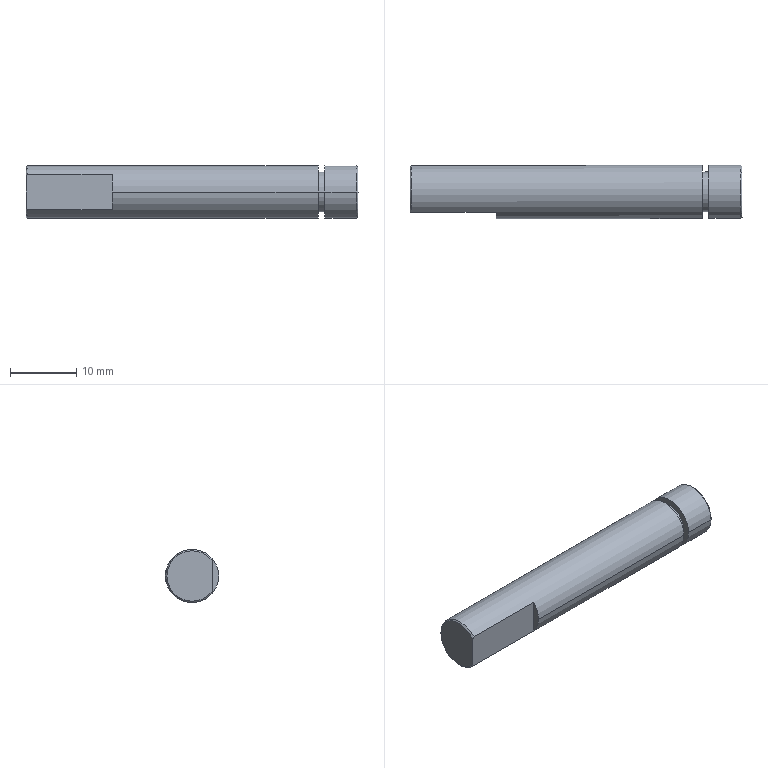Part | SolidWorks | features BaseBody 1 | 1 solid | 15 faces | box 50.007 x 8.035 x 8 mm | volume 2443 mm3 | cylinder 6 | plane 6 | cone 3 | commonest cylinder face diameters 8 x4 6 x2
STEP:
#1=CARTESIAN_POINT('',(349.379,469.971,106.919));
#2=VERTEX_POINT('',#1);
#3=CARTESIAN_POINT('',(349.387,461.971,106.919));
#4=VERTEX_POINT('',#3);
#5=CARTESIAN_POINT('',(349.383,465.971,106.919));
#6=DIRECTION('',(-1.,-0.0009599,0.));
#7=DIRECTION('',(0.0009599,-1.,0.));
#8=AXIS2_PLACEMENT_3D('',#5,#6,#7);
#9=CIRCLE('',#8,4.);
#10=EDGE_CURVE('',#2,#4,#9,.T.);
#11=ORIENTED_EDGE('',*,*,#10,.F.);
#12=CARTESIAN_POINT('',(354.179,469.976,106.919));
#13=VERTEX_POINT('',#12);
#14=CARTESIAN_POINT('',(304.379,469.928,106.919));
#15=DIRECTION('',(1.,0.0009599,0.));
#16=VECTOR('',#15,1000.);
#17=LINE('',#14,#16);
#18=EDGE_CURVE('',#2,#13,#17,.T.);
#19=ORIENTED_EDGE('',*,*,#18,.T.);
#20=CARTESIAN_POINT('',(354.187,461.976,106.919));
#21=VERTEX_POINT('',#20);
#22=CARTESIAN_POINT('',(354.183,465.976,106.919));
#23=DIRECTION('',(1.,0.0009599,0.));
#24=DIRECTION('',(-0.0009599,1.,0.));
#25=AXIS2_PLACEMENT_3D('',#22,#23,#24);
#26=CIRCLE('',#25,4.);
#27=EDGE_CURVE('',#21,#13,#26,.T.);
#28=ORIENTED_EDGE('',*,*,#27,.F.);
#29=CARTESIAN_POINT('',(304.387,461.928,106.919));
#30=DIRECTION('',(1.,0.0009599,0.));
#31=VECTOR('',#30,1000.);
#32=LINE('',#29,#31);
#33=EDGE_CURVE('',#4,#21,#32,.T.);
#34=ORIENTED_EDGE('',*,*,#33,.F.);
#35=EDGE_LOOP('',(#11,#19,#28,#34));
#36=FACE_OUTER_BOUND('',#35,.T.);
#37=CARTESIAN_POINT('',(304.383,465.928,106.919));
#38=DIRECTION('',(1.,0.0009599,0.));
#39=DIRECTION('',(0.0009599,-1.,0.));
#40=AXIS2_PLACEMENT_3D('',#37,#38,#39);
#41=CYLINDRICAL_SURFACE('',#40,4.);
#42=ADVANCED_FACE('',(#36),#41,.T.);
#43=CARTESIAN_POINT('',(348.38,468.97,106.919));
#44=VERTEX_POINT('',#43);
#45=CARTESIAN_POINT('',(348.386,462.97,106.919));
#46=VERTEX_POINT('',#45);
#47=CARTESIAN_POINT('',(348.383,465.97,106.919));
#48=DIRECTION('',(-1.,-0.0009599,0.));
#49=DIRECTION('',(-0.0009599,1.,0.));
#50=AXIS2_PLACEMENT_3D('',#47,#48,#49);
#51=CIRCLE('',#50,3.);
#52=EDGE_CURVE('',#44,#46,#51,.T.);
#53=ORIENTED_EDGE('',*,*,#52,.F.);
#54=CARTESIAN_POINT('',(349.38,468.971,106.919));
#55=VERTEX_POINT('',#54);
#56=CARTESIAN_POINT('',(354.38,468.976,106.919));
#57=DIRECTION('',(1.,0.0009599,0.));
#58=VECTOR('',#57,1000.);
#59=LINE('',#56,#58);
#60=EDGE_CURVE('',#44,#55,#59,.T.);
#61=ORIENTED_EDGE('',*,*,#60,.T.);
#62=CARTESIAN_POINT('',(349.386,462.971,106.919));
#63=VERTEX_POINT('',#62);
#64=CARTESIAN_POINT('',(349.383,465.971,106.919));
#65=DIRECTION('',(1.,0.0009599,0.));
#66=DIRECTION('',(-0.0009599,1.,0.));
#67=AXIS2_PLACEMENT_3D('',#64,#65,#66);
#68=CIRCLE('',#67,3.);
#69=EDGE_CURVE('',#63,#55,#68,.T.);
#70=ORIENTED_EDGE('',*,*,#69,.F.);
#71=CARTESIAN_POINT('',(354.386,462.976,106.919));
#72=DIRECTION('',(1.,0.0009599,0.));
#73=VECTOR('',#72,1000.);
#74=LINE('',#71,#73);
#75=EDGE_CURVE('',#46,#63,#74,.T.);
#76=ORIENTED_EDGE('',*,*,#75,.F.);
#77=EDGE_LOOP('',(#53,#61,#70,#76));
#78=FACE_OUTER_BOUND('',#77,.T.);
#79=CARTESIAN_POINT('',(354.383,465.976,106.919));
#80=DIRECTION('',(1.,0.0009599,0.));
#81=DIRECTION('',(0.0009599,-1.,0.));
#82=AXIS2_PLACEMENT_3D('',#79,#80,#81);
#83=CYLINDRICAL_SURFACE('',#82,3.);
#84=ADVANCED_FACE('',(#78),#83,.T.);
#85=CARTESIAN_POINT('',(304.579,469.928,106.919));
#86=VERTEX_POINT('',#85);
#87=CARTESIAN_POINT('',(304.586,462.928,104.273));
#88=VERTEX_POINT('',#87);
#89=CARTESIAN_POINT('',(304.583,465.928,106.919));
#90=DIRECTION('',(-1.,-0.0009599,0.));
#91=DIRECTION('',(-0.0009599,1.,0.));
#92=AXIS2_PLACEMENT_3D('',#89,#90,#91);
#93=CIRCLE('',#92,4.);
#94=EDGE_CURVE('',#86,#88,#93,.T.);
#95=ORIENTED_EDGE('',*,*,#94,.F.);
#96=CARTESIAN_POINT('',(348.379,469.97,106.919));
#97=VERTEX_POINT('',#96);
#98=CARTESIAN_POINT('',(304.379,469.928,106.919));
#99=DIRECTION('',(1.,0.0009599,0.));
#100=VECTOR('',#99,1000.);
#101=LINE('',#98,#100);
#102=EDGE_CURVE('',#86,#97,#101,.T.);
#103=ORIENTED_EDGE('',*,*,#102,.T.);
#104=CARTESIAN_POINT('',(348.387,461.97,106.919));
#105=VERTEX_POINT('',#104);
#106=CARTESIAN_POINT('',(348.383,465.97,106.919));
#107=DIRECTION('',(1.,0.0009599,0.));
#108=DIRECTION('',(-0.0009599,1.,0.));
#109=AXIS2_PLACEMENT_3D('',#106,#107,#108);
#110=CIRCLE('',#109,4.);
#111=EDGE_CURVE('',#105,#97,#110,.T.);
#112=ORIENTED_EDGE('',*,*,#111,.F.);
#113=CARTESIAN_POINT('',(317.387,461.941,106.919));
#114=VERTEX_POINT('',#113);
#115=CARTESIAN_POINT('',(304.387,461.928,106.919));
#116=DIRECTION('',(1.,0.0009599,0.));
#117=VECTOR('',#116,1000.);
#118=LINE('',#115,#117);
#119=EDGE_CURVE('',#114,#105,#118,.T.);
#120=ORIENTED_EDGE('',*,*,#119,.F.);
#121=CARTESIAN_POINT('',(317.386,462.941,104.273));
#122=VERTEX_POINT('',#121);
#123=CARTESIAN_POINT('',(317.383,465.941,106.919));
#124=DIRECTION('',(-1.,-0.0009599,0.));
#125=DIRECTION('',(0.0007199,-0.75,-0.6614));
#126=AXIS2_PLACEMENT_3D('',#123,#124,#125);
#127=CIRCLE('',#126,4.);
#128=EDGE_CURVE('',#122,#114,#127,.T.);
#129=ORIENTED_EDGE('',*,*,#128,.F.);
#130=CARTESIAN_POINT('',(317.386,462.941,104.273));
#131=DIRECTION('',(-1.,-0.0009599,0.));
#132=VECTOR('',#131,1000.);
#133=LINE('',#130,#132);
#134=EDGE_CURVE('',#122,#88,#133,.T.);
#135=ORIENTED_EDGE('',*,*,#134,.T.);
#136=EDGE_LOOP('',(#95,#103,#112,#120,#129,#135));
#137=FACE_OUTER_BOUND('',#136,.T.);
#138=CARTESIAN_POINT('',(304.383,465.928,106.919));
#139=DIRECTION('',(1.,0.0009599,0.));
#140=DIRECTION('',(0.0009599,-1.,0.));
#141=AXIS2_PLACEMENT_3D('',#138,#139,#140);
#142=CYLINDRICAL_SURFACE('',#141,4.);
#143=ADVANCED_FACE('',(#137),#142,.T.);
#144=CARTESIAN_POINT('',(354.386,462.176,106.919));
#145=VERTEX_POINT('',#144);
#146=CARTESIAN_POINT('',(354.379,469.776,106.919));
#147=VERTEX_POINT('',#146);
#148=CARTESIAN_POINT('',(354.383,465.976,106.919));
#149=DIRECTION('',(1.,0.0009599,0.));
#150=DIRECTION('',(0.0009599,-1.,0.));
#151=AXIS2_PLACEMENT_3D('',#148,#149,#150);
#152=CIRCLE('',#151,3.8);
#153=EDGE_CURVE('',#145,#147,#152,.T.);
#154=ORIENTED_EDGE('',*,*,#153,.F.);
#155=CARTESIAN_POINT('',(354.286,462.076,106.919));
#156=DIRECTION('',(-0.7064,-0.7078,0.));
#157=VECTOR('',#156,1000.);
#158=LINE('',#155,#157);
#159=EDGE_CURVE('',#145,#21,#158,.T.);
#160=ORIENTED_EDGE('',*,*,#159,.T.);
#161=ORIENTED_EDGE('',*,*,#27,.T.);
#162=CARTESIAN_POINT('',(354.279,469.876,106.919));
#163=DIRECTION('',(-0.7078,0.7064,0.));
#164=VECTOR('',#163,1000.);
#165=LINE('',#162,#164);
#166=EDGE_CURVE('',#147,#13,#165,.T.);
#167=ORIENTED_EDGE('',*,*,#166,.F.);
#168=EDGE_LOOP('',(#154,#160,#161,#167));
#169=FACE_OUTER_BOUND('',#168,.T.);
#170=CARTESIAN_POINT('',(354.283,465.976,106.919));
#171=DIRECTION('',(-1.,-0.0009599,0.));
#172=DIRECTION('',(-0.0009599,1.,0.));
#173=AXIS2_PLACEMENT_3D('',#170,#171,#172);
#174=CONICAL_SURFACE('',#173,3.9,0.7854);
#175=ADVANCED_FACE('',(#169),#174,.T.);
#176=CARTESIAN_POINT('',(354.383,465.976,106.919));
#177=DIRECTION('',(1.,0.0009599,0.));
#178=DIRECTION('',(0.0009599,-1.,0.));
#179=AXIS2_PLACEMENT_3D('',#176,#177,#178);
#180=CIRCLE('',#179,3.8);
#181=EDGE_CURVE('',#147,#145,#180,.T.);
#182=ORIENTED_EDGE('',*,*,#181,.T.);
#183=ORIENTED_EDGE('',*,*,#153,.T.);
#184=EDGE_LOOP('',(#182,#183));
#185=FACE_OUTER_BOUND('',#184,.T.);
#186=CARTESIAN_POINT('',(354.383,465.976,106.919));
#187=DIRECTION('',(-1.,-0.0009599,0.));
#188=DIRECTION('',(-0.0009599,1.,0.));
#189=AXIS2_PLACEMENT_3D('',#186,#187,#188);
#190=PLANE('',#189);
#191=ADVANCED_FACE('',(#185),#190,.F.);
#192=ORIENTED_EDGE('',*,*,#159,.F.);
#193=ORIENTED_EDGE('',*,*,#181,.F.);
#194=ORIENTED_EDGE('',*,*,#166,.T.);
#195=CARTESIAN_POINT('',(354.183,465.976,106.919));
#196=DIRECTION('',(1.,0.0009599,0.));
#197=DIRECTION('',(-0.0009599,1.,0.));
#198=AXIS2_PLACEMENT_3D('',#195,#196,#197);
#199=CIRCLE('',#198,4.);
#200=EDGE_CURVE('',#13,#21,#199,.T.);
#201=ORIENTED_EDGE('',*,*,#200,.T.);
#202=EDGE_LOOP('',(#192,#193,#194,#201));
#203=FACE_OUTER_BOUND('',#202,.T.);
#204=CARTESIAN_POINT('',(354.283,465.976,106.919));
#205=DIRECTION('',(-1.,-0.0009599,0.));
#206=DIRECTION('',(-0.0009599,1.,0.));
#207=AXIS2_PLACEMENT_3D('',#204,#205,#206);
#208=CONICAL_SURFACE('',#207,3.9,0.7854);
#209=ADVANCED_FACE('',(#203),#208,.T.);
#210=ORIENTED_EDGE('',*,*,#128,.T.);
#211=CARTESIAN_POINT('',(317.386,462.941,109.565));
#212=VERTEX_POINT('',#211);
#213=CARTESIAN_POINT('',(317.383,465.941,106.919));
#214=DIRECTION('',(-1.,-0.0009599,0.));
#215=DIRECTION('',(0.0007199,-0.75,-0.6614));
#216=AXIS2_PLACEMENT_3D('',#213,#214,#215);
#217=CIRCLE('',#216,4.);
#218=EDGE_CURVE('',#114,#212,#217,.T.);
#219=ORIENTED_EDGE('',*,*,#218,.T.);
#220=CARTESIAN_POINT('',(317.386,462.941,104.273));
#221=DIRECTION('',(0.,0.,1.));
#222=VECTOR('',#221,1000.);
#223=LINE('',#220,#222);
#224=EDGE_CURVE('',#122,#212,#223,.T.);
#225=ORIENTED_EDGE('',*,*,#224,.F.);
#226=EDGE_LOOP('',(#210,#219,#225));
#227=FACE_OUTER_BOUND('',#226,.T.);
#228=CARTESIAN_POINT('',(317.383,465.941,106.919));
#229=DIRECTION('',(-1.,-0.0009599,0.));
#230=DIRECTION('',(-0.0009599,1.,0.));
#231=AXIS2_PLACEMENT_3D('',#228,#229,#230);
#232=PLANE('',#231);
#233=ADVANCED_FACE('',(#227),#232,.T.);
#234=CARTESIAN_POINT('',(304.386,462.928,109.252));
#235=VERTEX_POINT('',#234);
#236=CARTESIAN_POINT('',(304.386,462.928,104.587));
#237=VERTEX_POINT('',#236);
#238=CARTESIAN_POINT('',(304.383,465.928,106.919));
#239=DIRECTION('',(-1.,-0.0009599,0.));
#240=DIRECTION('',(0.0007578,-0.7895,0.6138));
#241=AXIS2_PLACEMENT_3D('',#238,#239,#240);
#242=CIRCLE('',#241,3.8);
#243=EDGE_CURVE('',#235,#237,#242,.T.);
#244=ORIENTED_EDGE('',*,*,#243,.T.);
#245=CARTESIAN_POINT('',(304.386,462.928,104.587));
#246=DIRECTION('',(0.,0.,1.));
#247=VECTOR('',#246,1000.);
#248=LINE('',#245,#247);
#249=EDGE_CURVE('',#237,#235,#248,.T.);
#250=ORIENTED_EDGE('',*,*,#249,.T.);
#251=EDGE_LOOP('',(#244,#250));
#252=FACE_OUTER_BOUND('',#251,.T.);
#253=CARTESIAN_POINT('',(304.383,465.928,106.919));
#254=DIRECTION('',(-1.,-0.0009599,0.));
#255=DIRECTION('',(-0.0009599,1.,0.));
#256=AXIS2_PLACEMENT_3D('',#253,#254,#255);
#257=PLANE('',#256);
#258=ADVANCED_FACE('',(#252),#257,.T.);
#259=CARTESIAN_POINT('',(304.586,462.928,104.273));
#260=CARTESIAN_POINT('',(304.562,462.928,104.308));
#261=CARTESIAN_POINT('',(304.517,462.928,104.378));
#262=CARTESIAN_POINT('',(304.45,462.928,104.483));
#263=CARTESIAN_POINT('',(304.407,462.928,104.552));
#264=CARTESIAN_POINT('',(304.386,462.928,104.587));
#265=B_SPLINE_CURVE_WITH_KNOTS('',3,(#259,#260,#261,#262,#263,#264),.UNSPECIFIED.,.F.,.F.,(4,1,1,4),(0.,0.3333,0.6667,1.),.UNSPECIFIED.);
#266=EDGE_CURVE('',#88,#237,#265,.T.);
#267=ORIENTED_EDGE('',*,*,#266,.F.);
#268=ORIENTED_EDGE('',*,*,#134,.F.);
#269=ORIENTED_EDGE('',*,*,#224,.T.);
#270=CARTESIAN_POINT('',(304.586,462.928,109.565));
#271=VERTEX_POINT('',#270);
#272=CARTESIAN_POINT('',(304.586,462.928,109.565));
#273=DIRECTION('',(1.,0.0009599,0.));
#274=VECTOR('',#273,1000.);
#275=LINE('',#272,#274);
#276=EDGE_CURVE('',#271,#212,#275,.T.);
#277=ORIENTED_EDGE('',*,*,#276,.F.);
#278=CARTESIAN_POINT('',(304.386,462.928,109.252));
#279=CARTESIAN_POINT('',(304.407,462.928,109.286));
#280=CARTESIAN_POINT('',(304.45,462.928,109.356));
#281=CARTESIAN_POINT('',(304.517,462.928,109.46));
#282=CARTESIAN_POINT('',(304.562,462.928,109.53));
#283=CARTESIAN_POINT('',(304.586,462.928,109.565));
#284=B_SPLINE_CURVE_WITH_KNOTS('',3,(#278,#279,#280,#281,#282,#283),.UNSPECIFIED.,.F.,.F.,(4,1,1,4),(0.,0.3333,0.6667,1.),.UNSPECIFIED.);
#285=EDGE_CURVE('',#235,#271,#284,.T.);
#286=ORIENTED_EDGE('',*,*,#285,.F.);
#287=ORIENTED_EDGE('',*,*,#249,.F.);
#288=EDGE_LOOP('',(#267,#268,#269,#277,#286,#287));
#289=FACE_OUTER_BOUND('',#288,.T.);
#290=CARTESIAN_POINT('',(240.306,462.867,109.565));
#291=DIRECTION('',(0.0009599,-1.,0.));
#292=DIRECTION('',(0.,0.,-1.));
#293=AXIS2_PLACEMENT_3D('',#290,#291,#292);
#294=PLANE('',#293);
#295=ADVANCED_FACE('',(#289),#294,.T.);
#296=ORIENTED_EDGE('',*,*,#285,.T.);
#297=CARTESIAN_POINT('',(304.583,465.928,106.919));
#298=DIRECTION('',(-1.,-0.0009599,0.));
#299=DIRECTION('',(-0.0009599,1.,0.));
#300=AXIS2_PLACEMENT_3D('',#297,#298,#299);
#301=CIRCLE('',#300,4.);
#302=EDGE_CURVE('',#271,#86,#301,.T.);
#303=ORIENTED_EDGE('',*,*,#302,.T.);
#304=ORIENTED_EDGE('',*,*,#94,.T.);
#305=ORIENTED_EDGE('',*,*,#266,.T.);
#306=ORIENTED_EDGE('',*,*,#243,.F.);
#307=EDGE_LOOP('',(#296,#303,#304,#305,#306));
#308=FACE_OUTER_BOUND('',#307,.T.);
#309=CARTESIAN_POINT('',(304.483,465.928,106.919));
#310=DIRECTION('',(1.,0.0009599,0.));
#311=DIRECTION('',(0.0009599,-1.,0.));
#312=AXIS2_PLACEMENT_3D('',#309,#310,#311);
#313=CONICAL_SURFACE('',#312,3.9,0.7854);
#314=ADVANCED_FACE('',(#308),#313,.T.);
#315=ORIENTED_EDGE('',*,*,#102,.F.);
#316=ORIENTED_EDGE('',*,*,#302,.F.);
#317=ORIENTED_EDGE('',*,*,#276,.T.);
#318=ORIENTED_EDGE('',*,*,#218,.F.);
#319=ORIENTED_EDGE('',*,*,#119,.T.);
#320=CARTESIAN_POINT('',(348.383,465.97,106.919));
#321=DIRECTION('',(1.,0.0009599,0.));
#322=DIRECTION('',(-0.0009599,1.,0.));
#323=AXIS2_PLACEMENT_3D('',#320,#321,#322);
#324=CIRCLE('',#323,4.);
#325=EDGE_CURVE('',#97,#105,#324,.T.);
#326=ORIENTED_EDGE('',*,*,#325,.F.);
#327=EDGE_LOOP('',(#315,#316,#317,#318,#319,#326));
#328=FACE_OUTER_BOUND('',#327,.T.);
#329=CARTESIAN_POINT('',(304.383,465.928,106.919));
#330=DIRECTION('',(1.,0.0009599,0.));
#331=DIRECTION('',(0.0009599,-1.,0.));
#332=AXIS2_PLACEMENT_3D('',#329,#330,#331);
#333=CYLINDRICAL_SURFACE('',#332,4.);
#334=ADVANCED_FACE('',(#328),#333,.T.);
#335=CARTESIAN_POINT('',(348.383,465.97,106.919));
#336=DIRECTION('',(-1.,-0.0009599,0.));
#337=DIRECTION('',(-0.0009599,1.,0.));
#338=AXIS2_PLACEMENT_3D('',#335,#336,#337);
#339=CIRCLE('',#338,3.);
#340=EDGE_CURVE('',#46,#44,#339,.T.);
#341=ORIENTED_EDGE('',*,*,#340,.T.);
#342=ORIENTED_EDGE('',*,*,#52,.T.);
#343=EDGE_LOOP('',(#341,#342));
#344=FACE_BOUND('',#343,.T.);
#345=ORIENTED_EDGE('',*,*,#111,.T.);
#346=ORIENTED_EDGE('',*,*,#325,.T.);
#347=EDGE_LOOP('',(#345,#346));
#348=FACE_OUTER_BOUND('',#347,.T.);
#349=CARTESIAN_POINT('',(348.387,461.97,106.919));
#350=DIRECTION('',(-1.,-0.0009599,0.));
#351=DIRECTION('',(-0.0009599,1.,0.));
#352=AXIS2_PLACEMENT_3D('',#349,#350,#351);
#353=PLANE('',#352);
#354=ADVANCED_FACE('',(#344,#348),#353,.F.);
#355=ORIENTED_EDGE('',*,*,#60,.F.);
#356=ORIENTED_EDGE('',*,*,#340,.F.);
#357=ORIENTED_EDGE('',*,*,#75,.T.);
#358=CARTESIAN_POINT('',(349.383,465.971,106.919));
#359=DIRECTION('',(1.,0.0009599,0.));
#360=DIRECTION('',(-0.0009599,1.,0.));
#361=AXIS2_PLACEMENT_3D('',#358,#359,#360);
#362=CIRCLE('',#361,3.);
#363=EDGE_CURVE('',#55,#63,#362,.T.);
#364=ORIENTED_EDGE('',*,*,#363,.F.);
#365=EDGE_LOOP('',(#355,#356,#357,#364));
#366=FACE_OUTER_BOUND('',#365,.T.);
#367=CARTESIAN_POINT('',(354.383,465.976,106.919));
#368=DIRECTION('',(1.,0.0009599,0.));
#369=DIRECTION('',(0.0009599,-1.,0.));
#370=AXIS2_PLACEMENT_3D('',#367,#368,#369);
#371=CYLINDRICAL_SURFACE('',#370,3.);
#372=ADVANCED_FACE('',(#366),#371,.T.);
#373=ORIENTED_EDGE('',*,*,#69,.T.);
#374=ORIENTED_EDGE('',*,*,#363,.T.);
#375=EDGE_LOOP('',(#373,#374));
#376=FACE_BOUND('',#375,.T.);
#377=CARTESIAN_POINT('',(349.383,465.971,106.919));
#378=DIRECTION('',(-1.,-0.0009599,0.));
#379=DIRECTION('',(0.0009599,-1.,0.));
#380=AXIS2_PLACEMENT_3D('',#377,#378,#379);
#381=CIRCLE('',#380,4.);
#382=EDGE_CURVE('',#4,#2,#381,.T.);
#383=ORIENTED_EDGE('',*,*,#382,.T.);
#384=ORIENTED_EDGE('',*,*,#10,.T.);
#385=EDGE_LOOP('',(#383,#384));
#386=FACE_OUTER_BOUND('',#385,.T.);
#387=CARTESIAN_POINT('',(349.387,461.971,106.919));
#388=DIRECTION('',(1.,0.0009599,0.));
#389=DIRECTION('',(0.,0.,-1.));
#390=AXIS2_PLACEMENT_3D('',#387,#388,#389);
#391=PLANE('',#390);
#392=ADVANCED_FACE('',(#376,#386),#391,.F.);
#393=ORIENTED_EDGE('',*,*,#18,.F.);
#394=ORIENTED_EDGE('',*,*,#382,.F.);
#395=ORIENTED_EDGE('',*,*,#33,.T.);
#396=ORIENTED_EDGE('',*,*,#200,.F.);
#397=EDGE_LOOP('',(#393,#394,#395,#396));
#398=FACE_OUTER_BOUND('',#397,.T.);
#399=CARTESIAN_POINT('',(304.383,465.928,106.919));
#400=DIRECTION('',(1.,0.0009599,0.));
#401=DIRECTION('',(0.0009599,-1.,0.));
#402=AXIS2_PLACEMENT_3D('',#399,#400,#401);
#403=CYLINDRICAL_SURFACE('',#402,4.);
#404=ADVANCED_FACE('',(#398),#403,.T.);
#405=CLOSED_SHELL('',(#42,#84,#143,#175,#191,#209,#233,#258,#295,#314,#334,#354,#372,#392,#404));
#406=MANIFOLD_SOLID_BREP('',#405);
#407=CARTESIAN_POINT('',(0.,0.,0.));
#408=DIRECTION('',(0.,0.,1.));
#409=DIRECTION('',(1.,0.,0.));
#410=AXIS2_PLACEMENT_3D('',#407,#408,#409);
#411=(LENGTH_UNIT()NAMED_UNIT(*)SI_UNIT(.MILLI.,.METRE.));
#412=UNCERTAINTY_MEASURE_WITH_UNIT(LENGTH_MEASURE(0.00001),#411,'','');
#413=(NAMED_UNIT(*)PLANE_ANGLE_UNIT()SI_UNIT($,.RADIAN.));
#414=(NAMED_UNIT(*)SI_UNIT($,.STERADIAN.)SOLID_ANGLE_UNIT());
#415=(GEOMETRIC_REPRESENTATION_CONTEXT(3)GLOBAL_UNCERTAINTY_ASSIGNED_CONTEXT((#412))GLOBAL_UNIT_ASSIGNED_CONTEXT((#411,#413,#414))REPRESENTATION_CONTEXT('',''));
#416=ADVANCED_BREP_SHAPE_REPRESENTATION('',(#406,#410),#415);